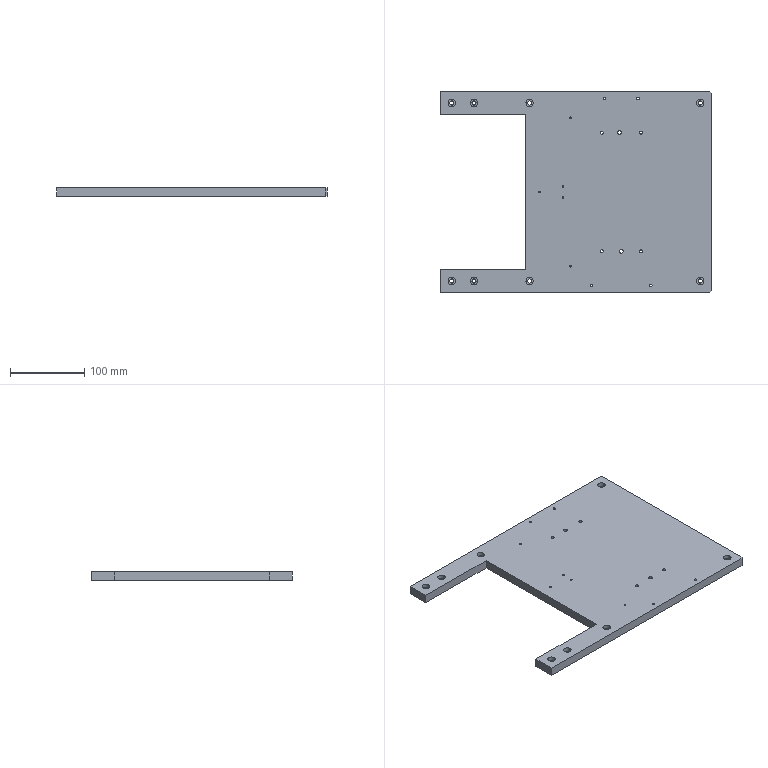CAM job | NX | 3-axis milling, drilling | part box 365 x 270 x 12 mm | stock box 369 x 274 x 13 mm
Tools:
number,name,description,diameter,corner_radius,flute_length,length,flutes
1,D50,Milling Tool-5 Parameters,50.0,0.0,50.0,75.0,2
2,D6A45,Milling Tool-5 Parameters,6.0,0.0,3.0,3.0,2
14,4.8ZT,Drilling Tool,4.8,0.0,35.0,50.0,2
16,5.0JD,Milling Tool-5 Parameters,5.0,0.0,30.0,30.0,4
15,5.5ZT,Drilling Tool,5.5,0.0,35.0,50.0,2
12,4.2ZT,Drilling Tool,4.2,0.0,35.0,50.0,2
13,3.3ZT,Drilling Tool,3.3,0.0,35.0,50.0,2
11,2.5ZT,Drilling Tool,2.5,0.0,35.0,50.0,2
8,D6,Milling Tool-5 Parameters,6.0,0.0,50.0,75.0,2
3,D10,Milling Tool-5 Parameters,10.0,0.0,50.0,75.0,2
6,D8JING,Milling Tool-5 Parameters,8.0,0.0,50.0,75.0,2
Operations:
program,operation,operation_type,tool,method,geometry_group,spindle_rpm,surface_speed,feed_per_tooth,feed_cut,feed_plunge,cut_length_mm,path_length_mm,cut_time_min,machine_time_min
1-368-272-12AB胶,FLOOR_WALL,VolumeBased25DMillingOperation,D50,METHOD,A,6500.0,1286.0,0.0962,1250.0,100.0,5293.997,5347.997,4.235,4.241
1-368-272-12AB胶,DRILLING_COPY_1,Operation,D6A45,METHOD,A,3000.0,56.0,0.0333,200.0,0.0,92.0,1555.01,0.46,0.6063
1-368-272-12AB胶,DRILLING_COPY_1_COPY_COPY_COPY_COPY_COPY_COPY_1_COPY_1,Operation,4.8ZT,METHOD,A,2000.0,20.0,0.0375,150.0,0.0,35.884,294.816,0.2392,0.2651
1-368-272-12AB胶,DRILLING_COPY_1_COPY_COPY_COPY_COPY_COPY_COPY_1_COPY_1_COPY,Operation,5.0JD,METHOD,A,1000.0,15.0,0.01,40.0,0.0,31.0,285.048,0.775,0.8004
1-368-272-12AB胶,DRILLING_COPY_1_COPY_COPY_COPY_COPY_COPY_COPY,Operation,5.5ZT,METHOD,A,2000.0,20.0,0.0375,150.0,0.0,145.219,1281.915,0.9681,1.082
1-368-272-12AB胶,DRILLING_COPY_1_COPY_COPY_COPY_COPY_1,Operation,4.2ZT,METHOD,A,2000.0,20.0,0.0375,150.0,0.0,67.047,469.292,0.447,0.4872
1-368-272-12AB胶,DRILLING_COPY_1_COPY_COPY_COPY_COPY_COPY,Operation,3.3ZT,METHOD,A,2000.0,20.0,0.0375,150.0,0.0,69.966,586.712,0.4664,0.5181
1-368-272-12AB胶,DRILLING_COPY_1_COPY_COPY_COPY_COPY_COPY_COPY_1,Operation,2.5ZT,METHOD,A,2000.0,20.0,0.0375,120.0,0.0,56.255,434.402,0.4688,0.5066
1-368-272-12AB胶,HOLE_MILLING,CylinderMilling,D6,METHOD,A,7000.0,131.0,0.1071,1500.0,100.0,1634.379,3063.579,1.09,1.232
1-368-272-12AB胶,ZLEVEL_PROFILE,ZLevelMilling,D10,METHOD,A,7000.0,219.0,0.2143,3000.0,1000.0,18406.708,18475.108,6.167,6.174
1-368-272-12AB胶,ZLEVEL_PROFILE_COPY_COPY_1_COPY_COPY_COPY_1_COPY_COPY_1,ZLevelMilling,D8JING,METHOD,A,7000.0,131.0,0.1071,1500.0,100.0,249.47,687.395,0.1663,0.2101
1-368-272-12AB胶,ZLEVEL_PROFILE_COPY_1_COPY_COPY_COPY_COPY_2_COPY,ZLevelMilling,D6A45,METHOD,A,7000.0,131.0,0.0714,1000.0,1000.0,1841.324,6021.952,1.841,2.259
1-368-272-12AB胶,ZLEVEL_PROFILE_COPY_1_1,ZLevelMilling,D8JING,METHOD,A,7000.0,219.0,0.0714,1000.0,1000.0,4570.304,4651.904,4.57,4.579